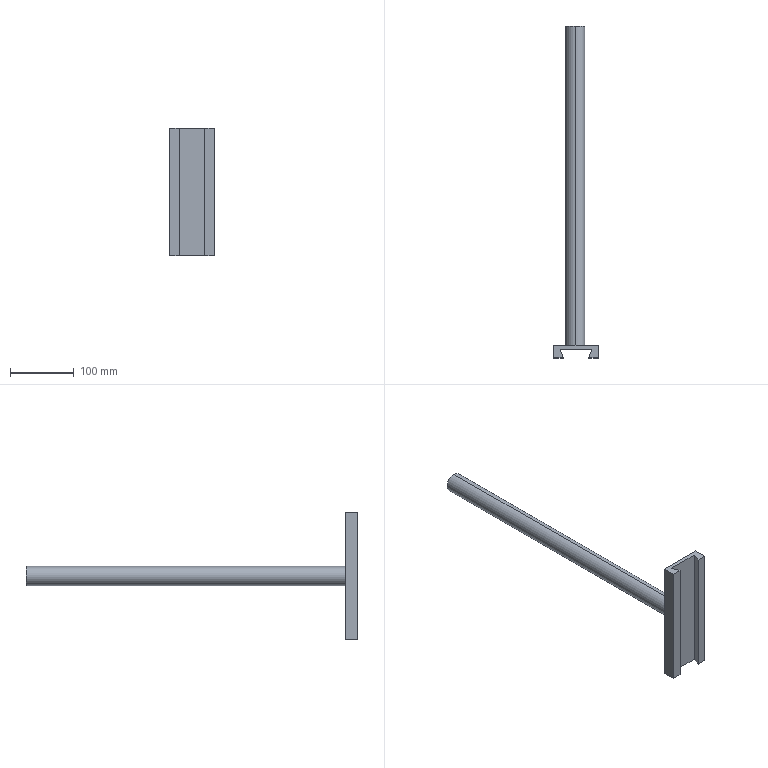Part | SolidWorks | features Extrusion 1, ICE 1 | 1 solid | 13 faces | box 70 x 520 x 200 mm | volume 509793 mm3 | plane 11 | cylinder 2 | commonest cylinder face diameters 30 x2
STEP:
#1=CARTESIAN_POINT('',(3.524,519.219,115.));
#2=VERTEX_POINT('',#1);
#3=CARTESIAN_POINT('',(3.524,519.219,85.));
#4=VERTEX_POINT('',#3);
#5=CARTESIAN_POINT('',(3.524,519.219,100.));
#6=DIRECTION('',(0.,1.,0.));
#7=DIRECTION('',(0.,0.,1.));
#8=AXIS2_PLACEMENT_3D('',#5,#6,#7);
#9=CIRCLE('',#8,15.);
#10=EDGE_CURVE('',#2,#4,#9,.T.);
#11=ORIENTED_EDGE('',*,*,#10,.F.);
#12=CARTESIAN_POINT('',(3.524,19.219,115.));
#13=VERTEX_POINT('',#12);
#14=CARTESIAN_POINT('',(3.524,519.219,115.));
#15=DIRECTION('',(0.,-1.,0.));
#16=VECTOR('',#15,1000.);
#17=LINE('',#14,#16);
#18=EDGE_CURVE('',#2,#13,#17,.T.);
#19=ORIENTED_EDGE('',*,*,#18,.T.);
#20=CARTESIAN_POINT('',(3.524,19.219,85.));
#21=VERTEX_POINT('',#20);
#22=CARTESIAN_POINT('',(3.524,19.219,100.));
#23=DIRECTION('',(0.,1.,0.));
#24=DIRECTION('',(0.,0.,-1.));
#25=AXIS2_PLACEMENT_3D('',#22,#23,#24);
#26=CIRCLE('',#25,15.);
#27=EDGE_CURVE('',#13,#21,#26,.T.);
#28=ORIENTED_EDGE('',*,*,#27,.T.);
#29=CARTESIAN_POINT('',(3.524,519.219,85.));
#30=DIRECTION('',(0.,-1.,0.));
#31=VECTOR('',#30,1000.);
#32=LINE('',#29,#31);
#33=EDGE_CURVE('',#4,#21,#32,.T.);
#34=ORIENTED_EDGE('',*,*,#33,.F.);
#35=EDGE_LOOP('',(#11,#19,#28,#34));
#36=FACE_OUTER_BOUND('',#35,.T.);
#37=CARTESIAN_POINT('',(3.524,519.219,100.));
#38=DIRECTION('',(0.,-1.,0.));
#39=DIRECTION('',(0.,0.,-1.));
#40=AXIS2_PLACEMENT_3D('',#37,#38,#39);
#41=CYLINDRICAL_SURFACE('',#40,15.);
#42=ADVANCED_FACE('',(#36),#41,.T.);
#43=CARTESIAN_POINT('',(39.738,19.219,0.));
#44=VERTEX_POINT('',#43);
#45=CARTESIAN_POINT('',(-30.262,19.219,0.));
#46=VERTEX_POINT('',#45);
#47=CARTESIAN_POINT('',(-30.262,19.219,0.));
#48=DIRECTION('',(-1.,0.,0.));
#49=VECTOR('',#48,1000.);
#50=LINE('',#47,#49);
#51=EDGE_CURVE('',#44,#46,#50,.T.);
#52=ORIENTED_EDGE('',*,*,#51,.T.);
#53=CARTESIAN_POINT('',(-30.262,19.219,200.));
#54=VERTEX_POINT('',#53);
#55=CARTESIAN_POINT('',(-30.262,19.219,200.));
#56=DIRECTION('',(0.,0.,-1.));
#57=VECTOR('',#56,1000.);
#58=LINE('',#55,#57);
#59=EDGE_CURVE('',#54,#46,#58,.T.);
#60=ORIENTED_EDGE('',*,*,#59,.F.);
#61=CARTESIAN_POINT('',(39.738,19.219,200.));
#62=VERTEX_POINT('',#61);
#63=CARTESIAN_POINT('',(-30.262,19.219,200.));
#64=DIRECTION('',(-1.,0.,0.));
#65=VECTOR('',#64,1000.);
#66=LINE('',#63,#65);
#67=EDGE_CURVE('',#62,#54,#66,.T.);
#68=ORIENTED_EDGE('',*,*,#67,.F.);
#69=CARTESIAN_POINT('',(39.738,19.219,200.));
#70=DIRECTION('',(0.,0.,-1.));
#71=VECTOR('',#70,1000.);
#72=LINE('',#69,#71);
#73=EDGE_CURVE('',#62,#44,#72,.T.);
#74=ORIENTED_EDGE('',*,*,#73,.T.);
#75=EDGE_LOOP('',(#52,#60,#68,#74));
#76=FACE_OUTER_BOUND('',#75,.T.);
#77=CARTESIAN_POINT('',(3.524,19.219,100.));
#78=DIRECTION('',(0.,1.,0.));
#79=DIRECTION('',(0.,0.,-1.));
#80=AXIS2_PLACEMENT_3D('',#77,#78,#79);
#81=CIRCLE('',#80,15.);
#82=EDGE_CURVE('',#21,#13,#81,.T.);
#83=ORIENTED_EDGE('',*,*,#82,.F.);
#84=ORIENTED_EDGE('',*,*,#27,.F.);
#85=EDGE_LOOP('',(#83,#84));
#86=FACE_BOUND('',#85,.T.);
#87=CARTESIAN_POINT('',(-30.262,19.219,200.));
#88=DIRECTION('',(0.,-1.,0.));
#89=DIRECTION('',(0.,0.,-1.));
#90=AXIS2_PLACEMENT_3D('',#87,#88,#89);
#91=PLANE('',#90);
#92=ADVANCED_FACE('',(#76,#86),#91,.F.);
#93=CARTESIAN_POINT('',(-30.262,-0.7809,0.));
#94=VERTEX_POINT('',#93);
#95=CARTESIAN_POINT('',(-30.262,-0.7809,0.));
#96=DIRECTION('',(0.,-1.,0.));
#97=VECTOR('',#96,1000.);
#98=LINE('',#95,#97);
#99=EDGE_CURVE('',#46,#94,#98,.T.);
#100=ORIENTED_EDGE('',*,*,#99,.T.);
#101=CARTESIAN_POINT('',(-30.262,-0.7809,200.));
#102=VERTEX_POINT('',#101);
#103=CARTESIAN_POINT('',(-30.262,-0.7809,200.));
#104=DIRECTION('',(0.,0.,-1.));
#105=VECTOR('',#104,1000.);
#106=LINE('',#103,#105);
#107=EDGE_CURVE('',#102,#94,#106,.T.);
#108=ORIENTED_EDGE('',*,*,#107,.F.);
#109=CARTESIAN_POINT('',(-30.262,-0.7809,200.));
#110=DIRECTION('',(0.,-1.,0.));
#111=VECTOR('',#110,1000.);
#112=LINE('',#109,#111);
#113=EDGE_CURVE('',#54,#102,#112,.T.);
#114=ORIENTED_EDGE('',*,*,#113,.F.);
#115=ORIENTED_EDGE('',*,*,#59,.T.);
#116=EDGE_LOOP('',(#100,#108,#114,#115));
#117=FACE_OUTER_BOUND('',#116,.T.);
#118=CARTESIAN_POINT('',(-30.262,-0.7809,200.));
#119=DIRECTION('',(1.,0.,0.));
#120=DIRECTION('',(0.,1.,0.));
#121=AXIS2_PLACEMENT_3D('',#118,#119,#120);
#122=PLANE('',#121);
#123=ADVANCED_FACE('',(#117),#122,.F.);
#124=CARTESIAN_POINT('',(-15.262,-0.7809,0.));
#125=VERTEX_POINT('',#124);
#126=CARTESIAN_POINT('',(-15.262,-0.7809,0.));
#127=DIRECTION('',(1.,0.,0.));
#128=VECTOR('',#127,1000.);
#129=LINE('',#126,#128);
#130=EDGE_CURVE('',#94,#125,#129,.T.);
#131=ORIENTED_EDGE('',*,*,#130,.T.);
#132=CARTESIAN_POINT('',(-15.262,-0.7809,200.));
#133=VERTEX_POINT('',#132);
#134=CARTESIAN_POINT('',(-15.262,-0.7809,200.));
#135=DIRECTION('',(0.,0.,-1.));
#136=VECTOR('',#135,1000.);
#137=LINE('',#134,#136);
#138=EDGE_CURVE('',#133,#125,#137,.T.);
#139=ORIENTED_EDGE('',*,*,#138,.F.);
#140=CARTESIAN_POINT('',(-15.262,-0.7809,200.));
#141=DIRECTION('',(1.,0.,0.));
#142=VECTOR('',#141,1000.);
#143=LINE('',#140,#142);
#144=EDGE_CURVE('',#102,#133,#143,.T.);
#145=ORIENTED_EDGE('',*,*,#144,.F.);
#146=ORIENTED_EDGE('',*,*,#107,.T.);
#147=EDGE_LOOP('',(#131,#139,#145,#146));
#148=FACE_OUTER_BOUND('',#147,.T.);
#149=CARTESIAN_POINT('',(-15.262,-0.7809,200.));
#150=DIRECTION('',(0.,1.,0.));
#151=DIRECTION('',(-1.,0.,0.));
#152=AXIS2_PLACEMENT_3D('',#149,#150,#151);
#153=PLANE('',#152);
#154=ADVANCED_FACE('',(#148),#153,.F.);
#155=CARTESIAN_POINT('',(-20.262,12.956,0.));
#156=VERTEX_POINT('',#155);
#157=CARTESIAN_POINT('',(-20.262,12.956,0.));
#158=DIRECTION('',(-0.342,0.9397,0.));
#159=VECTOR('',#158,1000.);
#160=LINE('',#157,#159);
#161=EDGE_CURVE('',#125,#156,#160,.T.);
#162=ORIENTED_EDGE('',*,*,#161,.T.);
#163=CARTESIAN_POINT('',(-20.262,12.956,200.));
#164=VERTEX_POINT('',#163);
#165=CARTESIAN_POINT('',(-20.262,12.956,200.));
#166=DIRECTION('',(0.,0.,-1.));
#167=VECTOR('',#166,1000.);
#168=LINE('',#165,#167);
#169=EDGE_CURVE('',#164,#156,#168,.T.);
#170=ORIENTED_EDGE('',*,*,#169,.F.);
#171=CARTESIAN_POINT('',(-20.262,12.956,200.));
#172=DIRECTION('',(-0.342,0.9397,0.));
#173=VECTOR('',#172,1000.);
#174=LINE('',#171,#173);
#175=EDGE_CURVE('',#133,#164,#174,.T.);
#176=ORIENTED_EDGE('',*,*,#175,.F.);
#177=ORIENTED_EDGE('',*,*,#138,.T.);
#178=EDGE_LOOP('',(#162,#170,#176,#177));
#179=FACE_OUTER_BOUND('',#178,.T.);
#180=CARTESIAN_POINT('',(-20.262,12.956,200.));
#181=DIRECTION('',(-0.9397,-0.342,0.));
#182=DIRECTION('',(0.342,-0.9397,0.));
#183=AXIS2_PLACEMENT_3D('',#180,#181,#182);
#184=PLANE('',#183);
#185=ADVANCED_FACE('',(#179),#184,.F.);
#186=CARTESIAN_POINT('',(29.738,12.956,0.));
#187=VERTEX_POINT('',#186);
#188=CARTESIAN_POINT('',(29.738,12.956,0.));
#189=DIRECTION('',(1.,0.,0.));
#190=VECTOR('',#189,1000.);
#191=LINE('',#188,#190);
#192=EDGE_CURVE('',#156,#187,#191,.T.);
#193=ORIENTED_EDGE('',*,*,#192,.T.);
#194=CARTESIAN_POINT('',(29.738,12.956,200.));
#195=VERTEX_POINT('',#194);
#196=CARTESIAN_POINT('',(29.738,12.956,200.));
#197=DIRECTION('',(0.,0.,-1.));
#198=VECTOR('',#197,1000.);
#199=LINE('',#196,#198);
#200=EDGE_CURVE('',#195,#187,#199,.T.);
#201=ORIENTED_EDGE('',*,*,#200,.F.);
#202=CARTESIAN_POINT('',(29.738,12.956,200.));
#203=DIRECTION('',(1.,0.,0.));
#204=VECTOR('',#203,1000.);
#205=LINE('',#202,#204);
#206=EDGE_CURVE('',#164,#195,#205,.T.);
#207=ORIENTED_EDGE('',*,*,#206,.F.);
#208=ORIENTED_EDGE('',*,*,#169,.T.);
#209=EDGE_LOOP('',(#193,#201,#207,#208));
#210=FACE_OUTER_BOUND('',#209,.T.);
#211=CARTESIAN_POINT('',(29.738,12.956,200.));
#212=DIRECTION('',(0.,1.,0.));
#213=DIRECTION('',(0.,0.,1.));
#214=AXIS2_PLACEMENT_3D('',#211,#212,#213);
#215=PLANE('',#214);
#216=ADVANCED_FACE('',(#210),#215,.F.);
#217=CARTESIAN_POINT('',(24.738,-0.7809,0.));
#218=VERTEX_POINT('',#217);
#219=CARTESIAN_POINT('',(24.738,-0.7809,0.));
#220=DIRECTION('',(-0.342,-0.9397,0.));
#221=VECTOR('',#220,1000.);
#222=LINE('',#219,#221);
#223=EDGE_CURVE('',#187,#218,#222,.T.);
#224=ORIENTED_EDGE('',*,*,#223,.T.);
#225=CARTESIAN_POINT('',(24.738,-0.7809,200.));
#226=VERTEX_POINT('',#225);
#227=CARTESIAN_POINT('',(24.738,-0.7809,200.));
#228=DIRECTION('',(0.,0.,-1.));
#229=VECTOR('',#228,1000.);
#230=LINE('',#227,#229);
#231=EDGE_CURVE('',#226,#218,#230,.T.);
#232=ORIENTED_EDGE('',*,*,#231,.F.);
#233=CARTESIAN_POINT('',(24.738,-0.7809,200.));
#234=DIRECTION('',(-0.342,-0.9397,0.));
#235=VECTOR('',#234,1000.);
#236=LINE('',#233,#235);
#237=EDGE_CURVE('',#195,#226,#236,.T.);
#238=ORIENTED_EDGE('',*,*,#237,.F.);
#239=ORIENTED_EDGE('',*,*,#200,.T.);
#240=EDGE_LOOP('',(#224,#232,#238,#239));
#241=FACE_OUTER_BOUND('',#240,.T.);
#242=CARTESIAN_POINT('',(24.738,-0.7809,200.));
#243=DIRECTION('',(0.9397,-0.342,0.));
#244=DIRECTION('',(0.342,0.9397,0.));
#245=AXIS2_PLACEMENT_3D('',#242,#243,#244);
#246=PLANE('',#245);
#247=ADVANCED_FACE('',(#241),#246,.F.);
#248=CARTESIAN_POINT('',(39.738,-0.7809,0.));
#249=VERTEX_POINT('',#248);
#250=CARTESIAN_POINT('',(39.738,-0.7809,0.));
#251=DIRECTION('',(1.,0.,0.));
#252=VECTOR('',#251,1000.);
#253=LINE('',#250,#252);
#254=EDGE_CURVE('',#218,#249,#253,.T.);
#255=ORIENTED_EDGE('',*,*,#254,.T.);
#256=CARTESIAN_POINT('',(39.738,-0.7809,200.));
#257=VERTEX_POINT('',#256);
#258=CARTESIAN_POINT('',(39.738,-0.7809,200.));
#259=DIRECTION('',(0.,0.,-1.));
#260=VECTOR('',#259,1000.);
#261=LINE('',#258,#260);
#262=EDGE_CURVE('',#257,#249,#261,.T.);
#263=ORIENTED_EDGE('',*,*,#262,.F.);
#264=CARTESIAN_POINT('',(39.738,-0.7809,200.));
#265=DIRECTION('',(1.,0.,0.));
#266=VECTOR('',#265,1000.);
#267=LINE('',#264,#266);
#268=EDGE_CURVE('',#226,#257,#267,.T.);
#269=ORIENTED_EDGE('',*,*,#268,.F.);
#270=ORIENTED_EDGE('',*,*,#231,.T.);
#271=EDGE_LOOP('',(#255,#263,#269,#270));
#272=FACE_OUTER_BOUND('',#271,.T.);
#273=CARTESIAN_POINT('',(39.738,-0.7809,200.));
#274=DIRECTION('',(0.,1.,0.));
#275=DIRECTION('',(-1.,0.,0.));
#276=AXIS2_PLACEMENT_3D('',#273,#274,#275);
#277=PLANE('',#276);
#278=ADVANCED_FACE('',(#272),#277,.F.);
#279=CARTESIAN_POINT('',(39.738,19.219,0.));
#280=DIRECTION('',(0.,1.,0.));
#281=VECTOR('',#280,1000.);
#282=LINE('',#279,#281);
#283=EDGE_CURVE('',#249,#44,#282,.T.);
#284=ORIENTED_EDGE('',*,*,#283,.T.);
#285=ORIENTED_EDGE('',*,*,#73,.F.);
#286=CARTESIAN_POINT('',(39.738,19.219,200.));
#287=DIRECTION('',(0.,1.,0.));
#288=VECTOR('',#287,1000.);
#289=LINE('',#286,#288);
#290=EDGE_CURVE('',#257,#62,#289,.T.);
#291=ORIENTED_EDGE('',*,*,#290,.F.);
#292=ORIENTED_EDGE('',*,*,#262,.T.);
#293=EDGE_LOOP('',(#284,#285,#291,#292));
#294=FACE_OUTER_BOUND('',#293,.T.);
#295=CARTESIAN_POINT('',(39.738,19.219,200.));
#296=DIRECTION('',(-1.,0.,0.));
#297=DIRECTION('',(0.,-1.,0.));
#298=AXIS2_PLACEMENT_3D('',#295,#296,#297);
#299=PLANE('',#298);
#300=ADVANCED_FACE('',(#294),#299,.F.);
#301=ORIENTED_EDGE('',*,*,#113,.T.);
#302=ORIENTED_EDGE('',*,*,#144,.T.);
#303=ORIENTED_EDGE('',*,*,#175,.T.);
#304=ORIENTED_EDGE('',*,*,#206,.T.);
#305=ORIENTED_EDGE('',*,*,#237,.T.);
#306=ORIENTED_EDGE('',*,*,#268,.T.);
#307=ORIENTED_EDGE('',*,*,#290,.T.);
#308=ORIENTED_EDGE('',*,*,#67,.T.);
#309=EDGE_LOOP('',(#301,#302,#303,#304,#305,#306,#307,#308));
#310=FACE_OUTER_BOUND('',#309,.T.);
#311=CARTESIAN_POINT('',(0.,0.,200.));
#312=DIRECTION('',(0.,0.,-1.));
#313=DIRECTION('',(-1.,0.,0.));
#314=AXIS2_PLACEMENT_3D('',#311,#312,#313);
#315=PLANE('',#314);
#316=ADVANCED_FACE('',(#310),#315,.F.);
#317=ORIENTED_EDGE('',*,*,#99,.F.);
#318=ORIENTED_EDGE('',*,*,#51,.F.);
#319=ORIENTED_EDGE('',*,*,#283,.F.);
#320=ORIENTED_EDGE('',*,*,#254,.F.);
#321=ORIENTED_EDGE('',*,*,#223,.F.);
#322=ORIENTED_EDGE('',*,*,#192,.F.);
#323=ORIENTED_EDGE('',*,*,#161,.F.);
#324=ORIENTED_EDGE('',*,*,#130,.F.);
#325=EDGE_LOOP('',(#317,#318,#319,#320,#321,#322,#323,#324));
#326=FACE_OUTER_BOUND('',#325,.T.);
#327=CARTESIAN_POINT('',(0.,0.,0.));
#328=DIRECTION('',(0.,0.,-1.));
#329=DIRECTION('',(-1.,0.,0.));
#330=AXIS2_PLACEMENT_3D('',#327,#328,#329);
#331=PLANE('',#330);
#332=ADVANCED_FACE('',(#326),#331,.T.);
#333=ORIENTED_EDGE('',*,*,#18,.F.);
#334=CARTESIAN_POINT('',(3.524,519.219,100.));
#335=DIRECTION('',(0.,1.,0.));
#336=DIRECTION('',(0.,0.,1.));
#337=AXIS2_PLACEMENT_3D('',#334,#335,#336);
#338=CIRCLE('',#337,15.);
#339=EDGE_CURVE('',#4,#2,#338,.T.);
#340=ORIENTED_EDGE('',*,*,#339,.F.);
#341=ORIENTED_EDGE('',*,*,#33,.T.);
#342=ORIENTED_EDGE('',*,*,#82,.T.);
#343=EDGE_LOOP('',(#333,#340,#341,#342));
#344=FACE_OUTER_BOUND('',#343,.T.);
#345=CARTESIAN_POINT('',(3.524,519.219,100.));
#346=DIRECTION('',(0.,-1.,0.));
#347=DIRECTION('',(0.,0.,-1.));
#348=AXIS2_PLACEMENT_3D('',#345,#346,#347);
#349=CYLINDRICAL_SURFACE('',#348,15.);
#350=ADVANCED_FACE('',(#344),#349,.T.);
#351=ORIENTED_EDGE('',*,*,#339,.T.);
#352=ORIENTED_EDGE('',*,*,#10,.T.);
#353=EDGE_LOOP('',(#351,#352));
#354=FACE_OUTER_BOUND('',#353,.T.);
#355=CARTESIAN_POINT('',(3.524,519.219,100.));
#356=DIRECTION('',(0.,1.,0.));
#357=DIRECTION('',(0.,0.,1.));
#358=AXIS2_PLACEMENT_3D('',#355,#356,#357);
#359=PLANE('',#358);
#360=ADVANCED_FACE('',(#354),#359,.T.);
#361=CLOSED_SHELL('',(#42,#92,#123,#154,#185,#216,#247,#278,#300,#316,#332,#350,#360));
#362=MANIFOLD_SOLID_BREP('',#361);
#363=CARTESIAN_POINT('',(0.,0.,0.));
#364=DIRECTION('',(0.,0.,1.));
#365=DIRECTION('',(1.,0.,0.));
#366=AXIS2_PLACEMENT_3D('',#363,#364,#365);
#367=(LENGTH_UNIT()NAMED_UNIT(*)SI_UNIT(.MILLI.,.METRE.));
#368=UNCERTAINTY_MEASURE_WITH_UNIT(LENGTH_MEASURE(0.00001),#367,'','');
#369=(NAMED_UNIT(*)PLANE_ANGLE_UNIT()SI_UNIT($,.RADIAN.));
#370=(NAMED_UNIT(*)SI_UNIT($,.STERADIAN.)SOLID_ANGLE_UNIT());
#371=(GEOMETRIC_REPRESENTATION_CONTEXT(3)GLOBAL_UNCERTAINTY_ASSIGNED_CONTEXT((#368))GLOBAL_UNIT_ASSIGNED_CONTEXT((#367,#369,#370))REPRESENTATION_CONTEXT('',''));
#372=ADVANCED_BREP_SHAPE_REPRESENTATION('',(#362,#366),#371);